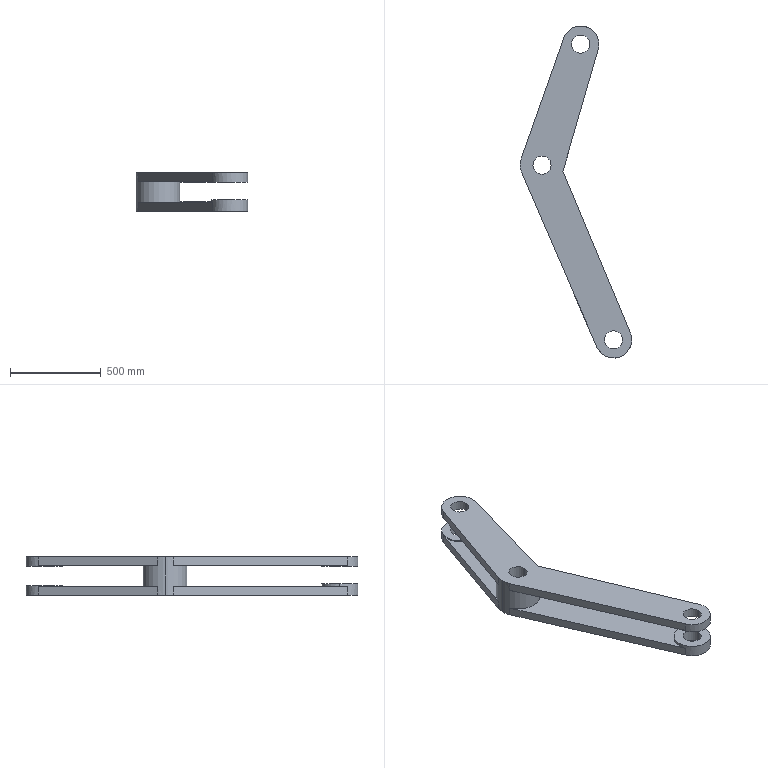Part | SolidWorks | features ICE 5, Extrusion 1 | 1 solid | 38 faces | box 614.266 x 1830 x 210 mm | volume 39335089 mm3 | cylinder 20 | plane 18 | commonest cylinder face diameters 100 x10 200 x8 240 x2
STEP:
#1=CARTESIAN_POINT('',(13655.596,320.325,-165.));
#2=VERTEX_POINT('',#1);
#3=CARTESIAN_POINT('',(13755.596,320.325,-165.));
#4=VERTEX_POINT('',#3);
#5=CARTESIAN_POINT('',(13705.596,320.325,-165.));
#6=DIRECTION('',(0.,0.,1.));
#7=DIRECTION('',(1.,0.,0.));
#8=AXIS2_PLACEMENT_3D('',#5,#6,#7);
#9=CIRCLE('',#8,50.);
#10=EDGE_CURVE('',#2,#4,#9,.T.);
#11=ORIENTED_EDGE('',*,*,#10,.F.);
#12=CARTESIAN_POINT('',(13655.596,320.325,-102.));
#13=VERTEX_POINT('',#12);
#14=CARTESIAN_POINT('',(13655.596,320.325,-165.));
#15=DIRECTION('',(0.,0.,1.));
#16=VECTOR('',#15,1000.);
#17=LINE('',#14,#16);
#18=EDGE_CURVE('',#2,#13,#17,.T.);
#19=ORIENTED_EDGE('',*,*,#18,.T.);
#20=CARTESIAN_POINT('',(13755.596,320.325,-102.));
#21=VERTEX_POINT('',#20);
#22=CARTESIAN_POINT('',(13705.596,320.325,-102.));
#23=DIRECTION('',(0.,0.,1.));
#24=DIRECTION('',(1.,0.,0.));
#25=AXIS2_PLACEMENT_3D('',#22,#23,#24);
#26=CIRCLE('',#25,50.);
#27=EDGE_CURVE('',#13,#21,#26,.T.);
#28=ORIENTED_EDGE('',*,*,#27,.T.);
#29=CARTESIAN_POINT('',(13755.596,320.325,-165.));
#30=DIRECTION('',(0.,0.,1.));
#31=VECTOR('',#30,1000.);
#32=LINE('',#29,#31);
#33=EDGE_CURVE('',#4,#21,#32,.T.);
#34=ORIENTED_EDGE('',*,*,#33,.F.);
#35=EDGE_LOOP('',(#11,#19,#28,#34));
#36=FACE_OUTER_BOUND('',#35,.T.);
#37=CARTESIAN_POINT('',(13705.596,320.325,-165.));
#38=DIRECTION('',(0.,0.,1.));
#39=DIRECTION('',(1.,0.,0.));
#40=AXIS2_PLACEMENT_3D('',#37,#38,#39);
#41=CYLINDRICAL_SURFACE('',#40,50.);
#42=ADVANCED_FACE('',(#36),#41,.F.);
#43=CARTESIAN_POINT('',(13474.67,1950.472,-165.));
#44=VERTEX_POINT('',#43);
#45=CARTESIAN_POINT('',(13574.67,1950.472,-165.));
#46=VERTEX_POINT('',#45);
#47=CARTESIAN_POINT('',(13524.67,1950.472,-165.));
#48=DIRECTION('',(0.,0.,1.));
#49=DIRECTION('',(1.,0.,0.));
#50=AXIS2_PLACEMENT_3D('',#47,#48,#49);
#51=CIRCLE('',#50,50.);
#52=EDGE_CURVE('',#44,#46,#51,.T.);
#53=ORIENTED_EDGE('',*,*,#52,.F.);
#54=CARTESIAN_POINT('',(13474.67,1950.472,-115.));
#55=VERTEX_POINT('',#54);
#56=CARTESIAN_POINT('',(13474.67,1950.472,-165.));
#57=DIRECTION('',(0.,0.,1.));
#58=VECTOR('',#57,1000.);
#59=LINE('',#56,#58);
#60=EDGE_CURVE('',#44,#55,#59,.T.);
#61=ORIENTED_EDGE('',*,*,#60,.T.);
#62=CARTESIAN_POINT('',(13574.67,1950.472,-115.));
#63=VERTEX_POINT('',#62);
#64=CARTESIAN_POINT('',(13524.67,1950.472,-115.));
#65=DIRECTION('',(0.,0.,1.));
#66=DIRECTION('',(1.,0.,0.));
#67=AXIS2_PLACEMENT_3D('',#64,#65,#66);
#68=CIRCLE('',#67,50.);
#69=EDGE_CURVE('',#55,#63,#68,.T.);
#70=ORIENTED_EDGE('',*,*,#69,.T.);
#71=CARTESIAN_POINT('',(13574.67,1950.472,-165.));
#72=DIRECTION('',(0.,0.,1.));
#73=VECTOR('',#72,1000.);
#74=LINE('',#71,#73);
#75=EDGE_CURVE('',#46,#63,#74,.T.);
#76=ORIENTED_EDGE('',*,*,#75,.F.);
#77=EDGE_LOOP('',(#53,#61,#70,#76));
#78=FACE_OUTER_BOUND('',#77,.T.);
#79=CARTESIAN_POINT('',(13524.67,1950.472,-165.));
#80=DIRECTION('',(0.,0.,1.));
#81=DIRECTION('',(1.,0.,0.));
#82=AXIS2_PLACEMENT_3D('',#79,#80,#81);
#83=CYLINDRICAL_SURFACE('',#82,50.);
#84=ADVANCED_FACE('',(#78),#83,.F.);
#85=CARTESIAN_POINT('',(13797.913,358.764,-120.));
#86=VERTEX_POINT('',#85);
#87=CARTESIAN_POINT('',(13605.596,320.325,-120.));
#88=VERTEX_POINT('',#87);
#89=CARTESIAN_POINT('',(13705.596,320.325,-120.));
#90=DIRECTION('',(0.,0.,1.));
#91=DIRECTION('',(1.,0.,0.));
#92=AXIS2_PLACEMENT_3D('',#89,#90,#91);
#93=CIRCLE('',#92,100.);
#94=EDGE_CURVE('',#86,#88,#93,.T.);
#95=ORIENTED_EDGE('',*,*,#94,.T.);
#96=CARTESIAN_POINT('',(13605.596,320.325,-102.));
#97=VERTEX_POINT('',#96);
#98=CARTESIAN_POINT('',(13605.596,320.325,-165.));
#99=DIRECTION('',(0.,0.,1.));
#100=VECTOR('',#99,1000.);
#101=LINE('',#98,#100);
#102=EDGE_CURVE('',#88,#97,#101,.T.);
#103=ORIENTED_EDGE('',*,*,#102,.T.);
#104=CARTESIAN_POINT('',(13805.596,320.325,-102.));
#105=VERTEX_POINT('',#104);
#106=CARTESIAN_POINT('',(13705.596,320.325,-102.));
#107=DIRECTION('',(0.,0.,1.));
#108=DIRECTION('',(1.,0.,0.));
#109=AXIS2_PLACEMENT_3D('',#106,#107,#108);
#110=CIRCLE('',#109,100.);
#111=EDGE_CURVE('',#105,#97,#110,.T.);
#112=ORIENTED_EDGE('',*,*,#111,.F.);
#113=CARTESIAN_POINT('',(13805.596,320.325,-165.));
#114=VERTEX_POINT('',#113);
#115=CARTESIAN_POINT('',(13805.596,320.325,-165.));
#116=DIRECTION('',(0.,0.,1.));
#117=VECTOR('',#116,1000.);
#118=LINE('',#115,#117);
#119=EDGE_CURVE('',#114,#105,#118,.T.);
#120=ORIENTED_EDGE('',*,*,#119,.F.);
#121=CARTESIAN_POINT('',(13797.913,358.764,-165.));
#122=VERTEX_POINT('',#121);
#123=CARTESIAN_POINT('',(13705.596,320.325,-165.));
#124=DIRECTION('',(0.,0.,1.));
#125=DIRECTION('',(1.,0.,0.));
#126=AXIS2_PLACEMENT_3D('',#123,#124,#125);
#127=CIRCLE('',#126,100.);
#128=EDGE_CURVE('',#114,#122,#127,.T.);
#129=ORIENTED_EDGE('',*,*,#128,.T.);
#130=CARTESIAN_POINT('',(13797.913,358.764,-165.));
#131=DIRECTION('',(0.,0.,1.));
#132=VECTOR('',#131,1000.);
#133=LINE('',#130,#132);
#134=EDGE_CURVE('',#122,#86,#133,.T.);
#135=ORIENTED_EDGE('',*,*,#134,.T.);
#136=EDGE_LOOP('',(#95,#103,#112,#120,#129,#135));
#137=FACE_OUTER_BOUND('',#136,.T.);
#138=CARTESIAN_POINT('',(13705.596,320.325,-165.));
#139=DIRECTION('',(0.,0.,1.));
#140=DIRECTION('',(1.,0.,0.));
#141=AXIS2_PLACEMENT_3D('',#138,#139,#140);
#142=CYLINDRICAL_SURFACE('',#141,100.);
#143=ADVANCED_FACE('',(#137),#142,.T.);
#144=CARTESIAN_POINT('',(13430.338,1983.658,-120.));
#145=VERTEX_POINT('',#144);
#146=CARTESIAN_POINT('',(13424.67,1950.472,-120.));
#147=VERTEX_POINT('',#146);
#148=CARTESIAN_POINT('',(13524.67,1950.472,-120.));
#149=DIRECTION('',(0.,0.,1.));
#150=DIRECTION('',(1.,0.,0.));
#151=AXIS2_PLACEMENT_3D('',#148,#149,#150);
#152=CIRCLE('',#151,100.);
#153=EDGE_CURVE('',#145,#147,#152,.T.);
#154=ORIENTED_EDGE('',*,*,#153,.T.);
#155=CARTESIAN_POINT('',(13424.67,1950.472,-115.));
#156=VERTEX_POINT('',#155);
#157=CARTESIAN_POINT('',(13424.67,1950.472,-165.));
#158=DIRECTION('',(0.,0.,1.));
#159=VECTOR('',#158,1000.);
#160=LINE('',#157,#159);
#161=EDGE_CURVE('',#147,#156,#160,.T.);
#162=ORIENTED_EDGE('',*,*,#161,.T.);
#163=CARTESIAN_POINT('',(13624.67,1950.472,-115.));
#164=VERTEX_POINT('',#163);
#165=CARTESIAN_POINT('',(13524.67,1950.472,-115.));
#166=DIRECTION('',(0.,0.,1.));
#167=DIRECTION('',(1.,0.,0.));
#168=AXIS2_PLACEMENT_3D('',#165,#166,#167);
#169=CIRCLE('',#168,100.);
#170=EDGE_CURVE('',#164,#156,#169,.T.);
#171=ORIENTED_EDGE('',*,*,#170,.F.);
#172=CARTESIAN_POINT('',(13624.67,1950.472,-165.));
#173=VERTEX_POINT('',#172);
#174=CARTESIAN_POINT('',(13624.67,1950.472,-165.));
#175=DIRECTION('',(0.,0.,1.));
#176=VECTOR('',#175,1000.);
#177=LINE('',#174,#176);
#178=EDGE_CURVE('',#173,#164,#177,.T.);
#179=ORIENTED_EDGE('',*,*,#178,.F.);
#180=CARTESIAN_POINT('',(13430.338,1983.658,-165.));
#181=VERTEX_POINT('',#180);
#182=CARTESIAN_POINT('',(13524.67,1950.472,-165.));
#183=DIRECTION('',(0.,0.,1.));
#184=DIRECTION('',(1.,0.,0.));
#185=AXIS2_PLACEMENT_3D('',#182,#183,#184);
#186=CIRCLE('',#185,100.);
#187=EDGE_CURVE('',#173,#181,#186,.T.);
#188=ORIENTED_EDGE('',*,*,#187,.T.);
#189=CARTESIAN_POINT('',(13430.338,1983.658,-165.));
#190=DIRECTION('',(0.,0.,1.));
#191=VECTOR('',#190,1000.);
#192=LINE('',#189,#191);
#193=EDGE_CURVE('',#181,#145,#192,.T.);
#194=ORIENTED_EDGE('',*,*,#193,.T.);
#195=EDGE_LOOP('',(#154,#162,#171,#179,#188,#194));
#196=FACE_OUTER_BOUND('',#195,.T.);
#197=CARTESIAN_POINT('',(13524.67,1950.472,-165.));
#198=DIRECTION('',(0.,0.,1.));
#199=DIRECTION('',(1.,0.,0.));
#200=AXIS2_PLACEMENT_3D('',#197,#198,#199);
#201=CYLINDRICAL_SURFACE('',#200,100.);
#202=ADVANCED_FACE('',(#196),#201,.T.);
#203=CARTESIAN_POINT('',(13655.596,320.325,45.));
#204=VERTEX_POINT('',#203);
#205=CARTESIAN_POINT('',(13755.596,320.325,45.));
#206=VERTEX_POINT('',#205);
#207=CARTESIAN_POINT('',(13705.596,320.325,45.));
#208=DIRECTION('',(0.,0.,1.));
#209=DIRECTION('',(1.,0.,0.));
#210=AXIS2_PLACEMENT_3D('',#207,#208,#209);
#211=CIRCLE('',#210,50.);
#212=EDGE_CURVE('',#204,#206,#211,.T.);
#213=ORIENTED_EDGE('',*,*,#212,.T.);
#214=CARTESIAN_POINT('',(13755.596,320.325,-5.));
#215=VERTEX_POINT('',#214);
#216=CARTESIAN_POINT('',(13755.596,320.325,45.));
#217=DIRECTION('',(0.,0.,-1.));
#218=VECTOR('',#217,1000.);
#219=LINE('',#216,#218);
#220=EDGE_CURVE('',#206,#215,#219,.T.);
#221=ORIENTED_EDGE('',*,*,#220,.T.);
#222=CARTESIAN_POINT('',(13655.596,320.325,-5.));
#223=VERTEX_POINT('',#222);
#224=CARTESIAN_POINT('',(13705.596,320.325,-5.));
#225=DIRECTION('',(0.,0.,1.));
#226=DIRECTION('',(1.,0.,0.));
#227=AXIS2_PLACEMENT_3D('',#224,#225,#226);
#228=CIRCLE('',#227,50.);
#229=EDGE_CURVE('',#223,#215,#228,.T.);
#230=ORIENTED_EDGE('',*,*,#229,.F.);
#231=CARTESIAN_POINT('',(13655.596,320.325,45.));
#232=DIRECTION('',(0.,0.,-1.));
#233=VECTOR('',#232,1000.);
#234=LINE('',#231,#233);
#235=EDGE_CURVE('',#204,#223,#234,.T.);
#236=ORIENTED_EDGE('',*,*,#235,.F.);
#237=EDGE_LOOP('',(#213,#221,#230,#236));
#238=FACE_OUTER_BOUND('',#237,.T.);
#239=CARTESIAN_POINT('',(13705.596,320.325,45.));
#240=DIRECTION('',(0.,0.,-1.));
#241=DIRECTION('',(-1.,0.,0.));
#242=AXIS2_PLACEMENT_3D('',#239,#240,#241);
#243=CYLINDRICAL_SURFACE('',#242,50.);
#244=ADVANCED_FACE('',(#238),#243,.F.);
#245=CARTESIAN_POINT('',(13624.67,1950.472,45.));
#246=VERTEX_POINT('',#245);
#247=CARTESIAN_POINT('',(13430.338,1983.658,45.));
#248=VERTEX_POINT('',#247);
#249=CARTESIAN_POINT('',(13524.67,1950.472,45.));
#250=DIRECTION('',(0.,0.,1.));
#251=DIRECTION('',(1.,0.,0.));
#252=AXIS2_PLACEMENT_3D('',#249,#250,#251);
#253=CIRCLE('',#252,100.);
#254=EDGE_CURVE('',#246,#248,#253,.T.);
#255=ORIENTED_EDGE('',*,*,#254,.F.);
#256=CARTESIAN_POINT('',(13624.67,1950.472,-5.));
#257=VERTEX_POINT('',#256);
#258=CARTESIAN_POINT('',(13624.67,1950.472,45.));
#259=DIRECTION('',(0.,0.,-1.));
#260=VECTOR('',#259,1000.);
#261=LINE('',#258,#260);
#262=EDGE_CURVE('',#246,#257,#261,.T.);
#263=ORIENTED_EDGE('',*,*,#262,.T.);
#264=CARTESIAN_POINT('',(13424.67,1950.472,-5.));
#265=VERTEX_POINT('',#264);
#266=CARTESIAN_POINT('',(13524.67,1950.472,-5.));
#267=DIRECTION('',(0.,0.,1.));
#268=DIRECTION('',(1.,0.,0.));
#269=AXIS2_PLACEMENT_3D('',#266,#267,#268);
#270=CIRCLE('',#269,100.);
#271=EDGE_CURVE('',#257,#265,#270,.T.);
#272=ORIENTED_EDGE('',*,*,#271,.T.);
#273=CARTESIAN_POINT('',(13424.67,1950.472,0.));
#274=VERTEX_POINT('',#273);
#275=CARTESIAN_POINT('',(13424.67,1950.472,45.));
#276=DIRECTION('',(0.,0.,-1.));
#277=VECTOR('',#276,1000.);
#278=LINE('',#275,#277);
#279=EDGE_CURVE('',#274,#265,#278,.T.);
#280=ORIENTED_EDGE('',*,*,#279,.F.);
#281=CARTESIAN_POINT('',(13430.338,1983.658,0.));
#282=VERTEX_POINT('',#281);
#283=CARTESIAN_POINT('',(13524.67,1950.472,0.));
#284=DIRECTION('',(0.,0.,1.));
#285=DIRECTION('',(1.,0.,0.));
#286=AXIS2_PLACEMENT_3D('',#283,#284,#285);
#287=CIRCLE('',#286,100.);
#288=EDGE_CURVE('',#282,#274,#287,.T.);
#289=ORIENTED_EDGE('',*,*,#288,.F.);
#290=CARTESIAN_POINT('',(13430.338,1983.658,45.));
#291=DIRECTION('',(0.,0.,-1.));
#292=VECTOR('',#291,1000.);
#293=LINE('',#290,#292);
#294=EDGE_CURVE('',#248,#282,#293,.T.);
#295=ORIENTED_EDGE('',*,*,#294,.F.);
#296=EDGE_LOOP('',(#255,#263,#272,#280,#289,#295));
#297=FACE_OUTER_BOUND('',#296,.T.);
#298=CARTESIAN_POINT('',(13524.67,1950.472,45.));
#299=DIRECTION('',(0.,0.,-1.));
#300=DIRECTION('',(-1.,0.,0.));
#301=AXIS2_PLACEMENT_3D('',#298,#299,#300);
#302=CYLINDRICAL_SURFACE('',#301,100.);
#303=ADVANCED_FACE('',(#297),#302,.T.);
#304=CARTESIAN_POINT('',(13474.67,1950.472,45.));
#305=VERTEX_POINT('',#304);
#306=CARTESIAN_POINT('',(13574.67,1950.472,45.));
#307=VERTEX_POINT('',#306);
#308=CARTESIAN_POINT('',(13524.67,1950.472,45.));
#309=DIRECTION('',(0.,0.,1.));
#310=DIRECTION('',(1.,0.,0.));
#311=AXIS2_PLACEMENT_3D('',#308,#309,#310);
#312=CIRCLE('',#311,50.);
#313=EDGE_CURVE('',#305,#307,#312,.T.);
#314=ORIENTED_EDGE('',*,*,#313,.T.);
#315=CARTESIAN_POINT('',(13574.67,1950.472,-5.));
#316=VERTEX_POINT('',#315);
#317=CARTESIAN_POINT('',(13574.67,1950.472,45.));
#318=DIRECTION('',(0.,0.,-1.));
#319=VECTOR('',#318,1000.);
#320=LINE('',#317,#319);
#321=EDGE_CURVE('',#307,#316,#320,.T.);
#322=ORIENTED_EDGE('',*,*,#321,.T.);
#323=CARTESIAN_POINT('',(13474.67,1950.472,-5.));
#324=VERTEX_POINT('',#323);
#325=CARTESIAN_POINT('',(13524.67,1950.472,-5.));
#326=DIRECTION('',(0.,0.,1.));
#327=DIRECTION('',(1.,0.,0.));
#328=AXIS2_PLACEMENT_3D('',#325,#326,#327);
#329=CIRCLE('',#328,50.);
#330=EDGE_CURVE('',#324,#316,#329,.T.);
#331=ORIENTED_EDGE('',*,*,#330,.F.);
#332=CARTESIAN_POINT('',(13474.67,1950.472,45.));
#333=DIRECTION('',(0.,0.,-1.));
#334=VECTOR('',#333,1000.);
#335=LINE('',#332,#334);
#336=EDGE_CURVE('',#305,#324,#335,.T.);
#337=ORIENTED_EDGE('',*,*,#336,.F.);
#338=EDGE_LOOP('',(#314,#322,#331,#337));
#339=FACE_OUTER_BOUND('',#338,.T.);
#340=CARTESIAN_POINT('',(13524.67,1950.472,45.));
#341=DIRECTION('',(0.,0.,-1.));
#342=DIRECTION('',(-1.,0.,0.));
#343=AXIS2_PLACEMENT_3D('',#340,#341,#342);
#344=CYLINDRICAL_SURFACE('',#343,50.);
#345=ADVANCED_FACE('',(#339),#344,.F.);
#346=CARTESIAN_POINT('',(13261.33,1283.774,45.));
#347=VERTEX_POINT('',#346);
#348=CARTESIAN_POINT('',(13361.33,1283.774,45.));
#349=VERTEX_POINT('',#348);
#350=CARTESIAN_POINT('',(13311.33,1283.774,45.));
#351=DIRECTION('',(0.,0.,1.));
#352=DIRECTION('',(1.,0.,0.));
#353=AXIS2_PLACEMENT_3D('',#350,#351,#352);
#354=CIRCLE('',#353,50.);
#355=EDGE_CURVE('',#347,#349,#354,.T.);
#356=ORIENTED_EDGE('',*,*,#355,.T.);
#357=CARTESIAN_POINT('',(13361.33,1283.774,-165.));
#358=VERTEX_POINT('',#357);
#359=CARTESIAN_POINT('',(13361.33,1283.774,45.));
#360=DIRECTION('',(0.,0.,-1.));
#361=VECTOR('',#360,1000.);
#362=LINE('',#359,#361);
#363=EDGE_CURVE('',#349,#358,#362,.T.);
#364=ORIENTED_EDGE('',*,*,#363,.T.);
#365=CARTESIAN_POINT('',(13261.33,1283.774,-165.));
#366=VERTEX_POINT('',#365);
#367=CARTESIAN_POINT('',(13311.33,1283.774,-165.));
#368=DIRECTION('',(0.,0.,1.));
#369=DIRECTION('',(1.,0.,0.));
#370=AXIS2_PLACEMENT_3D('',#367,#368,#369);
#371=CIRCLE('',#370,50.);
#372=EDGE_CURVE('',#366,#358,#371,.T.);
#373=ORIENTED_EDGE('',*,*,#372,.F.);
#374=CARTESIAN_POINT('',(13261.33,1283.774,45.));
#375=DIRECTION('',(0.,0.,-1.));
#376=VECTOR('',#375,1000.);
#377=LINE('',#374,#376);
#378=EDGE_CURVE('',#347,#366,#377,.T.);
#379=ORIENTED_EDGE('',*,*,#378,.F.);
#380=EDGE_LOOP('',(#356,#364,#373,#379));
#381=FACE_OUTER_BOUND('',#380,.T.);
#382=CARTESIAN_POINT('',(13311.33,1283.774,45.));
#383=DIRECTION('',(0.,0.,-1.));
#384=DIRECTION('',(-1.,0.,0.));
#385=AXIS2_PLACEMENT_3D('',#382,#383,#384);
#386=CYLINDRICAL_SURFACE('',#385,50.);
#387=ADVANCED_FACE('',(#381),#386,.F.);
#388=CARTESIAN_POINT('',(13805.596,320.325,45.));
#389=VERTEX_POINT('',#388);
#390=CARTESIAN_POINT('',(13797.913,358.764,45.));
#391=VERTEX_POINT('',#390);
#392=CARTESIAN_POINT('',(13705.596,320.325,45.));
#393=DIRECTION('',(0.,0.,1.));
#394=DIRECTION('',(1.,0.,0.));
#395=AXIS2_PLACEMENT_3D('',#392,#393,#394);
#396=CIRCLE('',#395,100.);
#397=EDGE_CURVE('',#389,#391,#396,.T.);
#398=ORIENTED_EDGE('',*,*,#397,.F.);
#399=CARTESIAN_POINT('',(13805.596,320.325,-5.));
#400=VERTEX_POINT('',#399);
#401=CARTESIAN_POINT('',(13805.596,320.325,45.));
#402=DIRECTION('',(0.,0.,-1.));
#403=VECTOR('',#402,1000.);
#404=LINE('',#401,#403);
#405=EDGE_CURVE('',#389,#400,#404,.T.);
#406=ORIENTED_EDGE('',*,*,#405,.T.);
#407=CARTESIAN_POINT('',(13605.596,320.325,-5.));
#408=VERTEX_POINT('',#407);
#409=CARTESIAN_POINT('',(13705.596,320.325,-5.));
#410=DIRECTION('',(0.,0.,1.));
#411=DIRECTION('',(1.,0.,0.));
#412=AXIS2_PLACEMENT_3D('',#409,#410,#411);
#413=CIRCLE('',#412,100.);
#414=EDGE_CURVE('',#400,#408,#413,.T.);
#415=ORIENTED_EDGE('',*,*,#414,.T.);
#416=CARTESIAN_POINT('',(13605.596,320.325,0.));
#417=VERTEX_POINT('',#416);
#418=CARTESIAN_POINT('',(13605.596,320.325,45.));
#419=DIRECTION('',(0.,0.,-1.));
#420=VECTOR('',#419,1000.);
#421=LINE('',#418,#420);
#422=EDGE_CURVE('',#417,#408,#421,.T.);
#423=ORIENTED_EDGE('',*,*,#422,.F.);
#424=CARTESIAN_POINT('',(13797.913,358.764,0.));
#425=VERTEX_POINT('',#424);
#426=CARTESIAN_POINT('',(13705.596,320.325,0.));
#427=DIRECTION('',(0.,0.,1.));
#428=DIRECTION('',(1.,0.,0.));
#429=AXIS2_PLACEMENT_3D('',#426,#427,#428);
#430=CIRCLE('',#429,100.);
#431=EDGE_CURVE('',#425,#417,#430,.T.);
#432=ORIENTED_EDGE('',*,*,#431,.F.);
#433=CARTESIAN_POINT('',(13797.913,358.764,45.));
#434=DIRECTION('',(0.,0.,-1.));
#435=VECTOR('',#434,1000.);
#436=LINE('',#433,#435);
#437=EDGE_CURVE('',#391,#425,#436,.T.);
#438=ORIENTED_EDGE('',*,*,#437,.F.);
#439=EDGE_LOOP('',(#398,#406,#415,#423,#432,#438));
#440=FACE_OUTER_BOUND('',#439,.T.);
#441=CARTESIAN_POINT('',(13705.596,320.325,45.));
#442=DIRECTION('',(0.,0.,-1.));
#443=DIRECTION('',(-1.,0.,0.));
#444=AXIS2_PLACEMENT_3D('',#441,#442,#443);
#445=CYLINDRICAL_SURFACE('',#444,100.);
#446=ADVANCED_FACE('',(#440),#445,.T.);
#447=CARTESIAN_POINT('',(13431.33,1283.774,0.));
#448=VERTEX_POINT('',#447);
#449=CARTESIAN_POINT('',(13198.13,1323.598,0.));
#450=VERTEX_POINT('',#449);
#451=CARTESIAN_POINT('',(13311.33,1283.774,0.));
#452=DIRECTION('',(0.,0.,1.));
#453=DIRECTION('',(1.,0.,0.));
#454=AXIS2_PLACEMENT_3D('',#451,#452,#453);
#455=CIRCLE('',#454,120.);
#456=EDGE_CURVE('',#448,#450,#455,.T.);
#457=ORIENTED_EDGE('',*,*,#456,.F.);
#458=CARTESIAN_POINT('',(13431.33,1283.774,-120.));
#459=VERTEX_POINT('',#458);
#460=CARTESIAN_POINT('',(13431.33,1283.774,45.));
#461=DIRECTION('',(0.,0.,-1.));
#462=VECTOR('',#461,1000.);
#463=LINE('',#460,#462);
#464=EDGE_CURVE('',#448,#459,#463,.T.);
#465=ORIENTED_EDGE('',*,*,#464,.T.);
#466=CARTESIAN_POINT('',(13198.13,1323.598,-120.));
#467=VERTEX_POINT('',#466);
#468=CARTESIAN_POINT('',(13311.33,1283.774,-120.));
#469=DIRECTION('',(0.,0.,1.));
#470=DIRECTION('',(1.,0.,0.));
#471=AXIS2_PLACEMENT_3D('',#468,#469,#470);
#472=CIRCLE('',#471,120.);
#473=EDGE_CURVE('',#459,#467,#472,.T.);
#474=ORIENTED_EDGE('',*,*,#473,.T.);
#475=CARTESIAN_POINT('',(13198.13,1323.598,-165.));
#476=VERTEX_POINT('',#475);
#477=CARTESIAN_POINT('',(13198.13,1323.598,-165.));
#478=DIRECTION('',(0.,0.,1.));
#479=VECTOR('',#478,1000.);
#480=LINE('',#477,#479);
#481=EDGE_CURVE('',#476,#467,#480,.T.);
#482=ORIENTED_EDGE('',*,*,#481,.F.);
#483=CARTESIAN_POINT('',(13191.33,1283.774,-165.));
#484=VERTEX_POINT('',#483);
#485=CARTESIAN_POINT('',(13311.33,1283.774,-165.));
#486=DIRECTION('',(0.,0.,1.));
#487=DIRECTION('',(1.,0.,0.));
#488=AXIS2_PLACEMENT_3D('',#485,#486,#487);
#489=CIRCLE('',#488,120.);
#490=EDGE_CURVE('',#476,#484,#489,.T.);
#491=ORIENTED_EDGE('',*,*,#490,.T.);
#492=CARTESIAN_POINT('',(13191.33,1283.774,45.));
#493=VERTEX_POINT('',#492);
#494=CARTESIAN_POINT('',(13191.33,1283.774,45.));
#495=DIRECTION('',(0.,0.,-1.));
#496=VECTOR('',#495,1000.);
#497=LINE('',#494,#496);
#498=EDGE_CURVE('',#493,#484,#497,.T.);
#499=ORIENTED_EDGE('',*,*,#498,.F.);
#500=CARTESIAN_POINT('',(13198.13,1323.598,45.));
#501=VERTEX_POINT('',#500);
#502=CARTESIAN_POINT('',(13311.33,1283.774,45.));
#503=DIRECTION('',(0.,0.,1.));
#504=DIRECTION('',(1.,0.,0.));
#505=AXIS2_PLACEMENT_3D('',#502,#503,#504);
#506=CIRCLE('',#505,120.);
#507=EDGE_CURVE('',#501,#493,#506,.T.);
#508=ORIENTED_EDGE('',*,*,#507,.F.);
#509=CARTESIAN_POINT('',(13198.13,1323.598,45.));
#510=DIRECTION('',(0.,0.,-1.));
#511=VECTOR('',#510,1000.);
#512=LINE('',#509,#511);
#513=EDGE_CURVE('',#501,#450,#512,.T.);
#514=ORIENTED_EDGE('',*,*,#513,.T.);
#515=EDGE_LOOP('',(#457,#465,#474,#482,#491,#499,#508,#514));
#516=FACE_OUTER_BOUND('',#515,.T.);
#517=CARTESIAN_POINT('',(13311.33,1283.774,45.));
#518=DIRECTION('',(0.,0.,-1.));
#519=DIRECTION('',(-1.,0.,0.));
#520=AXIS2_PLACEMENT_3D('',#517,#518,#519);
#521=CYLINDRICAL_SURFACE('',#520,120.);
#522=ADVANCED_FACE('',(#516),#521,.T.);
#523=CARTESIAN_POINT('',(13613.79,280.68,-120.));
#524=VERTEX_POINT('',#523);
#525=CARTESIAN_POINT('',(13201.163,1236.2,-120.));
#526=VERTEX_POINT('',#525);
#527=CARTESIAN_POINT('',(11576.243,4999.026,-120.));
#528=DIRECTION('',(-0.3964,0.9181,0.));
#529=VECTOR('',#528,1000.);
#530=LINE('',#527,#529);
#531=EDGE_CURVE('',#524,#526,#530,.T.);
#532=ORIENTED_EDGE('',*,*,#531,.F.);
#533=CARTESIAN_POINT('',(13705.596,320.325,-120.));
#534=DIRECTION('',(0.,0.,1.));
#535=DIRECTION('',(1.,0.,0.));
#536=AXIS2_PLACEMENT_3D('',#533,#534,#535);
#537=CIRCLE('',#536,100.);
#538=EDGE_CURVE('',#88,#524,#537,.T.);
#539=ORIENTED_EDGE('',*,*,#538,.F.);
#540=ORIENTED_EDGE('',*,*,#94,.F.);
#541=CARTESIAN_POINT('',(13426.619,1250.482,-120.));
#542=VERTEX_POINT('',#541);
#543=CARTESIAN_POINT('',(11886.503,4949.304,-120.));
#544=DIRECTION('',(0.3844,-0.9232,0.));
#545=VECTOR('',#544,1000.);
#546=LINE('',#543,#545);
#547=EDGE_CURVE('',#542,#86,#546,.T.);
#548=ORIENTED_EDGE('',*,*,#547,.F.);
#549=CARTESIAN_POINT('',(13311.33,1283.774,-120.));
#550=DIRECTION('',(0.,0.,1.));
#551=DIRECTION('',(1.,0.,0.));
#552=AXIS2_PLACEMENT_3D('',#549,#550,#551);
#553=CIRCLE('',#552,120.);
#554=EDGE_CURVE('',#526,#542,#553,.T.);
#555=ORIENTED_EDGE('',*,*,#554,.F.);
#556=EDGE_LOOP('',(#532,#539,#540,#548,#555));
#557=FACE_OUTER_BOUND('',#556,.T.);
#558=CARTESIAN_POINT('',(0.,0.,-120.));
#559=DIRECTION('',(0.,0.,1.));
#560=DIRECTION('',(1.,0.,0.));
#561=AXIS2_PLACEMENT_3D('',#558,#559,#560);
#562=PLANE('',#561);
#563=ADVANCED_FACE('',(#557),#562,.T.);
#564=CARTESIAN_POINT('',(13620.745,1922.728,-120.));
#565=VERTEX_POINT('',#564);
#566=CARTESIAN_POINT('',(12059.853,-3482.547,-120.));
#567=DIRECTION('',(-0.2774,-0.9607,0.));
#568=VECTOR('',#567,1000.);
#569=LINE('',#566,#568);
#570=EDGE_CURVE('',#565,#542,#569,.T.);
#571=ORIENTED_EDGE('',*,*,#570,.F.);
#572=CARTESIAN_POINT('',(13524.67,1950.472,-120.));
#573=DIRECTION('',(0.,0.,1.));
#574=DIRECTION('',(1.,0.,0.));
#575=AXIS2_PLACEMENT_3D('',#572,#573,#574);
#576=CIRCLE('',#575,100.);
#577=EDGE_CURVE('',#147,#565,#576,.T.);
#578=ORIENTED_EDGE('',*,*,#577,.F.);
#579=ORIENTED_EDGE('',*,*,#153,.F.);
#580=CARTESIAN_POINT('',(11330.248,-3985.948,-120.));
#581=DIRECTION('',(-0.3319,-0.9433,0.));
#582=VECTOR('',#581,1000.);
#583=LINE('',#580,#582);
#584=EDGE_CURVE('',#145,#467,#583,.T.);
#585=ORIENTED_EDGE('',*,*,#584,.T.);
#586=ORIENTED_EDGE('',*,*,#473,.F.);
#587=CARTESIAN_POINT('',(13311.33,1283.774,-120.));
#588=DIRECTION('',(0.,0.,1.));
#589=DIRECTION('',(1.,0.,0.));
#590=AXIS2_PLACEMENT_3D('',#587,#588,#589);
#591=CIRCLE('',#590,120.);
#592=EDGE_CURVE('',#542,#459,#591,.T.);
#593=ORIENTED_EDGE('',*,*,#592,.F.);
#594=EDGE_LOOP('',(#571,#578,#579,#585,#586,#593));
#595=FACE_OUTER_BOUND('',#594,.T.);
#596=CARTESIAN_POINT('',(0.,0.,-120.));
#597=DIRECTION('',(0.,0.,1.));
#598=DIRECTION('',(1.,0.,0.));
#599=AXIS2_PLACEMENT_3D('',#596,#597,#598);
#600=PLANE('',#599);
#601=ADVANCED_FACE('',(#595),#600,.T.);
#602=CARTESIAN_POINT('',(13426.619,1250.482,0.));
#603=VERTEX_POINT('',#602);
#604=CARTESIAN_POINT('',(11886.503,4949.304,0.));
#605=DIRECTION('',(0.3844,-0.9232,0.));
#606=VECTOR('',#605,1000.);
#607=LINE('',#604,#606);
#608=EDGE_CURVE('',#603,#425,#607,.T.);
#609=ORIENTED_EDGE('',*,*,#608,.T.);
#610=ORIENTED_EDGE('',*,*,#431,.T.);
#611=CARTESIAN_POINT('',(13613.79,280.68,0.));
#612=VERTEX_POINT('',#611);
#613=CARTESIAN_POINT('',(13705.596,320.325,0.));
#614=DIRECTION('',(0.,0.,1.));
#615=DIRECTION('',(1.,0.,0.));
#616=AXIS2_PLACEMENT_3D('',#613,#614,#615);
#617=CIRCLE('',#616,100.);
#618=EDGE_CURVE('',#417,#612,#617,.T.);
#619=ORIENTED_EDGE('',*,*,#618,.T.);
#620=CARTESIAN_POINT('',(13201.163,1236.2,0.));
#621=VERTEX_POINT('',#620);
#622=CARTESIAN_POINT('',(11576.243,4999.026,0.));
#623=DIRECTION('',(-0.3964,0.9181,0.));
#624=VECTOR('',#623,1000.);
#625=LINE('',#622,#624);
#626=EDGE_CURVE('',#612,#621,#625,.T.);
#627=ORIENTED_EDGE('',*,*,#626,.T.);
#628=CARTESIAN_POINT('',(13311.33,1283.774,0.));
#629=DIRECTION('',(0.,0.,1.));
#630=DIRECTION('',(1.,0.,0.));
#631=AXIS2_PLACEMENT_3D('',#628,#629,#630);
#632=CIRCLE('',#631,120.);
#633=EDGE_CURVE('',#621,#603,#632,.T.);
#634=ORIENTED_EDGE('',*,*,#633,.T.);
#635=EDGE_LOOP('',(#609,#610,#619,#627,#634));
#636=FACE_OUTER_BOUND('',#635,.T.);
#637=CARTESIAN_POINT('',(0.,0.,0.));
#638=DIRECTION('',(0.,0.,1.));
#639=DIRECTION('',(1.,0.,0.));
#640=AXIS2_PLACEMENT_3D('',#637,#638,#639);
#641=PLANE('',#640);
#642=ADVANCED_FACE('',(#636),#641,.F.);
#643=CARTESIAN_POINT('',(11330.248,-3985.948,0.));
#644=DIRECTION('',(-0.3319,-0.9433,0.));
#645=VECTOR('',#644,1000.);
#646=LINE('',#643,#645);
#647=EDGE_CURVE('',#282,#450,#646,.T.);
#648=ORIENTED_EDGE('',*,*,#647,.T.);
#649=ORIENTED_EDGE('',*,*,#513,.F.);
#650=CARTESIAN_POINT('',(11330.248,-3985.948,45.));
#651=DIRECTION('',(-0.3319,-0.9433,0.));
#652=VECTOR('',#651,1000.);
#653=LINE('',#650,#652);
#654=EDGE_CURVE('',#248,#501,#653,.T.);
#655=ORIENTED_EDGE('',*,*,#654,.F.);
#656=ORIENTED_EDGE('',*,*,#294,.T.);
#657=EDGE_LOOP('',(#648,#649,#655,#656));
#658=FACE_OUTER_BOUND('',#657,.T.);
#659=CARTESIAN_POINT('',(11330.248,-3985.948,45.));
#660=DIRECTION('',(0.9433,-0.3319,0.));
#661=DIRECTION('',(0.3319,0.9433,0.));
#662=AXIS2_PLACEMENT_3D('',#659,#660,#661);
#663=PLANE('',#662);
#664=ADVANCED_FACE('',(#658),#663,.F.);
#665=ORIENTED_EDGE('',*,*,#464,.F.);
#666=CARTESIAN_POINT('',(13311.33,1283.774,0.));
#667=DIRECTION('',(0.,0.,1.));
#668=DIRECTION('',(1.,0.,0.));
#669=AXIS2_PLACEMENT_3D('',#666,#667,#668);
#670=CIRCLE('',#669,120.);
#671=EDGE_CURVE('',#603,#448,#670,.T.);
#672=ORIENTED_EDGE('',*,*,#671,.F.);
#673=ORIENTED_EDGE('',*,*,#633,.F.);
#674=CARTESIAN_POINT('',(13201.163,1236.2,45.));
#675=VERTEX_POINT('',#674);
#676=CARTESIAN_POINT('',(13201.163,1236.2,45.));
#677=DIRECTION('',(0.,0.,-1.));
#678=VECTOR('',#677,1000.);
#679=LINE('',#676,#678);
#680=EDGE_CURVE('',#675,#621,#679,.T.);
#681=ORIENTED_EDGE('',*,*,#680,.F.);
#682=CARTESIAN_POINT('',(13311.33,1283.774,45.));
#683=DIRECTION('',(0.,0.,1.));
#684=DIRECTION('',(1.,0.,0.));
#685=AXIS2_PLACEMENT_3D('',#682,#683,#684);
#686=CIRCLE('',#685,120.);
#687=EDGE_CURVE('',#493,#675,#686,.T.);
#688=ORIENTED_EDGE('',*,*,#687,.F.);
#689=ORIENTED_EDGE('',*,*,#498,.T.);
#690=CARTESIAN_POINT('',(13201.163,1236.2,-165.));
#691=VERTEX_POINT('',#690);
#692=CARTESIAN_POINT('',(13311.33,1283.774,-165.));
#693=DIRECTION('',(0.,0.,1.));
#694=DIRECTION('',(1.,0.,0.));
#695=AXIS2_PLACEMENT_3D('',#692,#693,#694);
#696=CIRCLE('',#695,120.);
#697=EDGE_CURVE('',#484,#691,#696,.T.);
#698=ORIENTED_EDGE('',*,*,#697,.T.);
#699=CARTESIAN_POINT('',(13201.163,1236.2,-165.));
#700=DIRECTION('',(0.,0.,1.));
#701=VECTOR('',#700,1000.);
#702=LINE('',#699,#701);
#703=EDGE_CURVE('',#691,#526,#702,.T.);
#704=ORIENTED_EDGE('',*,*,#703,.T.);
#705=ORIENTED_EDGE('',*,*,#554,.T.);
#706=ORIENTED_EDGE('',*,*,#592,.T.);
#707=EDGE_LOOP('',(#665,#672,#673,#681,#688,#689,#698,#704,#705,#706));
#708=FACE_OUTER_BOUND('',#707,.T.);
#709=CARTESIAN_POINT('',(13311.33,1283.774,45.));
#710=DIRECTION('',(0.,0.,-1.));
#711=DIRECTION('',(-1.,0.,0.));
#712=AXIS2_PLACEMENT_3D('',#709,#710,#711);
#713=CYLINDRICAL_SURFACE('',#712,120.);
#714=ADVANCED_FACE('',(#708),#713,.T.);
#715=ORIENTED_EDGE('',*,*,#626,.F.);
#716=CARTESIAN_POINT('',(13613.79,280.68,45.));
#717=VERTEX_POINT('',#716);
#718=CARTESIAN_POINT('',(13613.79,280.68,45.));
#719=DIRECTION('',(0.,0.,-1.));
#720=VECTOR('',#719,1000.);
#721=LINE('',#718,#720);
#722=EDGE_CURVE('',#717,#612,#721,.T.);
#723=ORIENTED_EDGE('',*,*,#722,.F.);
#724=CARTESIAN_POINT('',(11576.243,4999.026,45.));
#725=DIRECTION('',(-0.3964,0.9181,0.));
#726=VECTOR('',#725,1000.);
#727=LINE('',#724,#726);
#728=EDGE_CURVE('',#717,#675,#727,.T.);
#729=ORIENTED_EDGE('',*,*,#728,.T.);
#730=ORIENTED_EDGE('',*,*,#680,.T.);
#731=EDGE_LOOP('',(#715,#723,#729,#730));
#732=FACE_OUTER_BOUND('',#731,.T.);
#733=CARTESIAN_POINT('',(11576.243,4999.026,45.));
#734=DIRECTION('',(-0.9181,-0.3964,0.));
#735=DIRECTION('',(0.3964,-0.9181,0.));
#736=AXIS2_PLACEMENT_3D('',#733,#734,#735);
#737=PLANE('',#736);
#738=ADVANCED_FACE('',(#732),#737,.T.);
#739=ORIENTED_EDGE('',*,*,#405,.F.);
#740=CARTESIAN_POINT('',(13705.596,320.325,45.));
#741=DIRECTION('',(0.,0.,1.));
#742=DIRECTION('',(1.,0.,0.));
#743=AXIS2_PLACEMENT_3D('',#740,#741,#742);
#744=CIRCLE('',#743,100.);
#745=EDGE_CURVE('',#717,#389,#744,.T.);
#746=ORIENTED_EDGE('',*,*,#745,.F.);
#747=ORIENTED_EDGE('',*,*,#722,.T.);
#748=ORIENTED_EDGE('',*,*,#618,.F.);
#749=ORIENTED_EDGE('',*,*,#422,.T.);
#750=CARTESIAN_POINT('',(13705.596,320.325,-5.));
#751=DIRECTION('',(0.,0.,1.));
#752=DIRECTION('',(1.,0.,0.));
#753=AXIS2_PLACEMENT_3D('',#750,#751,#752);
#754=CIRCLE('',#753,100.);
#755=EDGE_CURVE('',#408,#400,#754,.T.);
#756=ORIENTED_EDGE('',*,*,#755,.T.);
#757=EDGE_LOOP('',(#739,#746,#747,#748,#749,#756));
#758=FACE_OUTER_BOUND('',#757,.T.);
#759=CARTESIAN_POINT('',(13705.596,320.325,45.));
#760=DIRECTION('',(0.,0.,-1.));
#761=DIRECTION('',(-1.,0.,0.));
#762=AXIS2_PLACEMENT_3D('',#759,#760,#761);
#763=CYLINDRICAL_SURFACE('',#762,100.);
#764=ADVANCED_FACE('',(#758),#763,.T.);
#765=ORIENTED_EDGE('',*,*,#608,.F.);
#766=CARTESIAN_POINT('',(13426.619,1250.482,45.));
#767=VERTEX_POINT('',#766);
#768=CARTESIAN_POINT('',(13426.619,1250.482,45.));
#769=DIRECTION('',(0.,0.,-1.));
#770=VECTOR('',#769,1000.);
#771=LINE('',#768,#770);
#772=EDGE_CURVE('',#767,#603,#771,.T.);
#773=ORIENTED_EDGE('',*,*,#772,.F.);
#774=CARTESIAN_POINT('',(11886.503,4949.304,45.));
#775=DIRECTION('',(0.3844,-0.9232,0.));
#776=VECTOR('',#775,1000.);
#777=LINE('',#774,#776);
#778=EDGE_CURVE('',#767,#391,#777,.T.);
#779=ORIENTED_EDGE('',*,*,#778,.T.);
#780=ORIENTED_EDGE('',*,*,#437,.T.);
#781=EDGE_LOOP('',(#765,#773,#779,#780));
#782=FACE_OUTER_BOUND('',#781,.T.);
#783=CARTESIAN_POINT('',(11886.503,4949.304,45.));
#784=DIRECTION('',(0.9232,0.3844,0.));
#785=DIRECTION('',(-0.3844,0.9232,0.));
#786=AXIS2_PLACEMENT_3D('',#783,#784,#785);
#787=PLANE('',#786);
#788=ADVANCED_FACE('',(#782),#787,.T.);
#789=CARTESIAN_POINT('',(13620.745,1922.728,0.));
#790=VERTEX_POINT('',#789);
#791=CARTESIAN_POINT('',(12059.853,-3482.547,0.));
#792=DIRECTION('',(-0.2774,-0.9607,0.));
#793=VECTOR('',#792,1000.);
#794=LINE('',#791,#793);
#795=EDGE_CURVE('',#790,#603,#794,.T.);
#796=ORIENTED_EDGE('',*,*,#795,.F.);
#797=CARTESIAN_POINT('',(13620.745,1922.728,45.));
#798=VERTEX_POINT('',#797);
#799=CARTESIAN_POINT('',(13620.745,1922.728,45.));
#800=DIRECTION('',(0.,0.,-1.));
#801=VECTOR('',#800,1000.);
#802=LINE('',#799,#801);
#803=EDGE_CURVE('',#798,#790,#802,.T.);
#804=ORIENTED_EDGE('',*,*,#803,.F.);
#805=CARTESIAN_POINT('',(12059.853,-3482.547,45.));
#806=DIRECTION('',(-0.2774,-0.9607,0.));
#807=VECTOR('',#806,1000.);
#808=LINE('',#805,#807);
#809=EDGE_CURVE('',#798,#767,#808,.T.);
#810=ORIENTED_EDGE('',*,*,#809,.T.);
#811=ORIENTED_EDGE('',*,*,#772,.T.);
#812=EDGE_LOOP('',(#796,#804,#810,#811));
#813=FACE_OUTER_BOUND('',#812,.T.);
#814=CARTESIAN_POINT('',(12059.853,-3482.547,45.));
#815=DIRECTION('',(0.9607,-0.2774,0.));
#816=DIRECTION('',(0.2774,0.9607,0.));
#817=AXIS2_PLACEMENT_3D('',#814,#815,#816);
#818=PLANE('',#817);
#819=ADVANCED_FACE('',(#813),#818,.T.);
#820=ORIENTED_EDGE('',*,*,#363,.F.);
#821=CARTESIAN_POINT('',(13311.33,1283.774,45.));
#822=DIRECTION('',(0.,0.,1.));
#823=DIRECTION('',(1.,0.,0.));
#824=AXIS2_PLACEMENT_3D('',#821,#822,#823);
#825=CIRCLE('',#824,50.);
#826=EDGE_CURVE('',#349,#347,#825,.T.);
#827=ORIENTED_EDGE('',*,*,#826,.T.);
#828=ORIENTED_EDGE('',*,*,#378,.T.);
#829=CARTESIAN_POINT('',(13311.33,1283.774,-165.));
#830=DIRECTION('',(0.,0.,1.));
#831=DIRECTION('',(1.,0.,0.));
#832=AXIS2_PLACEMENT_3D('',#829,#830,#831);
#833=CIRCLE('',#832,50.);
#834=EDGE_CURVE('',#358,#366,#833,.T.);
#835=ORIENTED_EDGE('',*,*,#834,.F.);
#836=EDGE_LOOP('',(#820,#827,#828,#835));
#837=FACE_OUTER_BOUND('',#836,.T.);
#838=CARTESIAN_POINT('',(13311.33,1283.774,45.));
#839=DIRECTION('',(0.,0.,-1.));
#840=DIRECTION('',(-1.,0.,0.));
#841=AXIS2_PLACEMENT_3D('',#838,#839,#840);
#842=CYLINDRICAL_SURFACE('',#841,50.);
#843=ADVANCED_FACE('',(#837),#842,.F.);
#844=ORIENTED_EDGE('',*,*,#321,.F.);
#845=CARTESIAN_POINT('',(13524.67,1950.472,45.));
#846=DIRECTION('',(0.,0.,1.));
#847=DIRECTION('',(1.,0.,0.));
#848=AXIS2_PLACEMENT_3D('',#845,#846,#847);
#849=CIRCLE('',#848,50.);
#850=EDGE_CURVE('',#307,#305,#849,.T.);
#851=ORIENTED_EDGE('',*,*,#850,.T.);
#852=ORIENTED_EDGE('',*,*,#336,.T.);
#853=CARTESIAN_POINT('',(13524.67,1950.472,-5.));
#854=DIRECTION('',(0.,0.,1.));
#855=DIRECTION('',(1.,0.,0.));
#856=AXIS2_PLACEMENT_3D('',#853,#854,#855);
#857=CIRCLE('',#856,50.);
#858=EDGE_CURVE('',#316,#324,#857,.T.);
#859=ORIENTED_EDGE('',*,*,#858,.F.);
#860=EDGE_LOOP('',(#844,#851,#852,#859));
#861=FACE_OUTER_BOUND('',#860,.T.);
#862=CARTESIAN_POINT('',(13524.67,1950.472,45.));
#863=DIRECTION('',(0.,0.,-1.));
#864=DIRECTION('',(-1.,0.,0.));
#865=AXIS2_PLACEMENT_3D('',#862,#863,#864);
#866=CYLINDRICAL_SURFACE('',#865,50.);
#867=ADVANCED_FACE('',(#861),#866,.F.);
#868=ORIENTED_EDGE('',*,*,#262,.F.);
#869=CARTESIAN_POINT('',(13524.67,1950.472,45.));
#870=DIRECTION('',(0.,0.,1.));
#871=DIRECTION('',(1.,0.,0.));
#872=AXIS2_PLACEMENT_3D('',#869,#870,#871);
#873=CIRCLE('',#872,100.);
#874=EDGE_CURVE('',#798,#246,#873,.T.);
#875=ORIENTED_EDGE('',*,*,#874,.F.);
#876=ORIENTED_EDGE('',*,*,#803,.T.);
#877=CARTESIAN_POINT('',(13524.67,1950.472,0.));
#878=DIRECTION('',(0.,0.,1.));
#879=DIRECTION('',(1.,0.,0.));
#880=AXIS2_PLACEMENT_3D('',#877,#878,#879);
#881=CIRCLE('',#880,100.);
#882=EDGE_CURVE('',#274,#790,#881,.T.);
#883=ORIENTED_EDGE('',*,*,#882,.F.);
#884=ORIENTED_EDGE('',*,*,#279,.T.);
#885=CARTESIAN_POINT('',(13524.67,1950.472,-5.));
#886=DIRECTION('',(0.,0.,1.));
#887=DIRECTION('',(1.,0.,0.));
#888=AXIS2_PLACEMENT_3D('',#885,#886,#887);
#889=CIRCLE('',#888,100.);
#890=EDGE_CURVE('',#265,#257,#889,.T.);
#891=ORIENTED_EDGE('',*,*,#890,.T.);
#892=EDGE_LOOP('',(#868,#875,#876,#883,#884,#891));
#893=FACE_OUTER_BOUND('',#892,.T.);
#894=CARTESIAN_POINT('',(13524.67,1950.472,45.));
#895=DIRECTION('',(0.,0.,-1.));
#896=DIRECTION('',(-1.,0.,0.));
#897=AXIS2_PLACEMENT_3D('',#894,#895,#896);
#898=CYLINDRICAL_SURFACE('',#897,100.);
#899=ADVANCED_FACE('',(#893),#898,.T.);
#900=ORIENTED_EDGE('',*,*,#220,.F.);
#901=CARTESIAN_POINT('',(13705.596,320.325,45.));
#902=DIRECTION('',(0.,0.,1.));
#903=DIRECTION('',(1.,0.,0.));
#904=AXIS2_PLACEMENT_3D('',#901,#902,#903);
#905=CIRCLE('',#904,50.);
#906=EDGE_CURVE('',#206,#204,#905,.T.);
#907=ORIENTED_EDGE('',*,*,#906,.T.);
#908=ORIENTED_EDGE('',*,*,#235,.T.);
#909=CARTESIAN_POINT('',(13705.596,320.325,-5.));
#910=DIRECTION('',(0.,0.,1.));
#911=DIRECTION('',(1.,0.,0.));
#912=AXIS2_PLACEMENT_3D('',#909,#910,#911);
#913=CIRCLE('',#912,50.);
#914=EDGE_CURVE('',#215,#223,#913,.T.);
#915=ORIENTED_EDGE('',*,*,#914,.F.);
#916=EDGE_LOOP('',(#900,#907,#908,#915));
#917=FACE_OUTER_BOUND('',#916,.T.);
#918=CARTESIAN_POINT('',(13705.596,320.325,45.));
#919=DIRECTION('',(0.,0.,-1.));
#920=DIRECTION('',(-1.,0.,0.));
#921=AXIS2_PLACEMENT_3D('',#918,#919,#920);
#922=CYLINDRICAL_SURFACE('',#921,50.);
#923=ADVANCED_FACE('',(#917),#922,.F.);
#924=ORIENTED_EDGE('',*,*,#654,.T.);
#925=ORIENTED_EDGE('',*,*,#507,.T.);
#926=ORIENTED_EDGE('',*,*,#687,.T.);
#927=ORIENTED_EDGE('',*,*,#728,.F.);
#928=ORIENTED_EDGE('',*,*,#745,.T.);
#929=ORIENTED_EDGE('',*,*,#397,.T.);
#930=ORIENTED_EDGE('',*,*,#778,.F.);
#931=ORIENTED_EDGE('',*,*,#809,.F.);
#932=ORIENTED_EDGE('',*,*,#874,.T.);
#933=ORIENTED_EDGE('',*,*,#254,.T.);
#934=EDGE_LOOP('',(#924,#925,#926,#927,#928,#929,#930,#931,#932,#933));
#935=FACE_OUTER_BOUND('',#934,.T.);
#936=ORIENTED_EDGE('',*,*,#313,.F.);
#937=ORIENTED_EDGE('',*,*,#850,.F.);
#938=EDGE_LOOP('',(#936,#937));
#939=FACE_BOUND('',#938,.T.);
#940=ORIENTED_EDGE('',*,*,#355,.F.);
#941=ORIENTED_EDGE('',*,*,#826,.F.);
#942=EDGE_LOOP('',(#940,#941));
#943=FACE_BOUND('',#942,.T.);
#944=ORIENTED_EDGE('',*,*,#212,.F.);
#945=ORIENTED_EDGE('',*,*,#906,.F.);
#946=EDGE_LOOP('',(#944,#945));
#947=FACE_BOUND('',#946,.T.);
#948=CARTESIAN_POINT('',(0.,0.,45.));
#949=DIRECTION('',(0.,0.,1.));
#950=DIRECTION('',(1.,0.,0.));
#951=AXIS2_PLACEMENT_3D('',#948,#949,#950);
#952=PLANE('',#951);
#953=ADVANCED_FACE('',(#935,#939,#943,#947),#952,.T.);
#954=ORIENTED_EDGE('',*,*,#647,.F.);
#955=ORIENTED_EDGE('',*,*,#288,.T.);
#956=ORIENTED_EDGE('',*,*,#882,.T.);
#957=ORIENTED_EDGE('',*,*,#795,.T.);
#958=ORIENTED_EDGE('',*,*,#671,.T.);
#959=ORIENTED_EDGE('',*,*,#456,.T.);
#960=EDGE_LOOP('',(#954,#955,#956,#957,#958,#959));
#961=FACE_OUTER_BOUND('',#960,.T.);
#962=CARTESIAN_POINT('',(0.,0.,0.));
#963=DIRECTION('',(0.,0.,1.));
#964=DIRECTION('',(1.,0.,0.));
#965=AXIS2_PLACEMENT_3D('',#962,#963,#964);
#966=PLANE('',#965);
#967=ADVANCED_FACE('',(#961),#966,.F.);
#968=ORIENTED_EDGE('',*,*,#330,.T.);
#969=ORIENTED_EDGE('',*,*,#858,.T.);
#970=EDGE_LOOP('',(#968,#969));
#971=FACE_BOUND('',#970,.T.);
#972=ORIENTED_EDGE('',*,*,#890,.F.);
#973=ORIENTED_EDGE('',*,*,#271,.F.);
#974=EDGE_LOOP('',(#972,#973));
#975=FACE_OUTER_BOUND('',#974,.T.);
#976=CARTESIAN_POINT('',(0.,0.,-5.));
#977=DIRECTION('',(0.,0.,1.));
#978=DIRECTION('',(1.,0.,0.));
#979=AXIS2_PLACEMENT_3D('',#976,#977,#978);
#980=PLANE('',#979);
#981=ADVANCED_FACE('',(#971,#975),#980,.F.);
#982=ORIENTED_EDGE('',*,*,#229,.T.);
#983=ORIENTED_EDGE('',*,*,#914,.T.);
#984=EDGE_LOOP('',(#982,#983));
#985=FACE_BOUND('',#984,.T.);
#986=ORIENTED_EDGE('',*,*,#755,.F.);
#987=ORIENTED_EDGE('',*,*,#414,.F.);
#988=EDGE_LOOP('',(#986,#987));
#989=FACE_OUTER_BOUND('',#988,.T.);
#990=CARTESIAN_POINT('',(0.,0.,-5.));
#991=DIRECTION('',(0.,0.,1.));
#992=DIRECTION('',(1.,0.,0.));
#993=AXIS2_PLACEMENT_3D('',#990,#991,#992);
#994=PLANE('',#993);
#995=ADVANCED_FACE('',(#985,#989),#994,.F.);
#996=ORIENTED_EDGE('',*,*,#584,.F.);
#997=ORIENTED_EDGE('',*,*,#193,.F.);
#998=CARTESIAN_POINT('',(11330.248,-3985.948,-165.));
#999=DIRECTION('',(-0.3319,-0.9433,0.));
#1000=VECTOR('',#999,1000.);
#1001=LINE('',#998,#1000);
#1002=EDGE_CURVE('',#181,#476,#1001,.T.);
#1003=ORIENTED_EDGE('',*,*,#1002,.T.);
#1004=ORIENTED_EDGE('',*,*,#481,.T.);
#1005=EDGE_LOOP('',(#996,#997,#1003,#1004));
#1006=FACE_OUTER_BOUND('',#1005,.T.);
#1007=CARTESIAN_POINT('',(11330.248,-3985.948,-165.));
#1008=DIRECTION('',(-0.9433,0.3319,0.));
#1009=DIRECTION('',(-0.3319,-0.9433,0.));
#1010=AXIS2_PLACEMENT_3D('',#1007,#1008,#1009);
#1011=PLANE('',#1010);
#1012=ADVANCED_FACE('',(#1006),#1011,.T.);
#1013=ORIENTED_EDGE('',*,*,#161,.F.);
#1014=ORIENTED_EDGE('',*,*,#577,.T.);
#1015=CARTESIAN_POINT('',(13620.745,1922.728,-165.));
#1016=VERTEX_POINT('',#1015);
#1017=CARTESIAN_POINT('',(13620.745,1922.728,-165.));
#1018=DIRECTION('',(0.,0.,1.));
#1019=VECTOR('',#1018,1000.);
#1020=LINE('',#1017,#1019);
#1021=EDGE_CURVE('',#1016,#565,#1020,.T.);
#1022=ORIENTED_EDGE('',*,*,#1021,.F.);
#1023=CARTESIAN_POINT('',(13524.67,1950.472,-165.));
#1024=DIRECTION('',(0.,0.,1.));
#1025=DIRECTION('',(1.,0.,0.));
#1026=AXIS2_PLACEMENT_3D('',#1023,#1024,#1025);
#1027=CIRCLE('',#1026,100.);
#1028=EDGE_CURVE('',#1016,#173,#1027,.T.);
#1029=ORIENTED_EDGE('',*,*,#1028,.T.);
#1030=ORIENTED_EDGE('',*,*,#178,.T.);
#1031=CARTESIAN_POINT('',(13524.67,1950.472,-115.));
#1032=DIRECTION('',(0.,0.,1.));
#1033=DIRECTION('',(1.,0.,0.));
#1034=AXIS2_PLACEMENT_3D('',#1031,#1032,#1033);
#1035=CIRCLE('',#1034,100.);
#1036=EDGE_CURVE('',#156,#164,#1035,.T.);
#1037=ORIENTED_EDGE('',*,*,#1036,.F.);
#1038=EDGE_LOOP('',(#1013,#1014,#1022,#1029,#1030,#1037));
#1039=FACE_OUTER_BOUND('',#1038,.T.);
#1040=CARTESIAN_POINT('',(13524.67,1950.472,-165.));
#1041=DIRECTION('',(0.,0.,1.));
#1042=DIRECTION('',(1.,0.,0.));
#1043=AXIS2_PLACEMENT_3D('',#1040,#1041,#1042);
#1044=CYLINDRICAL_SURFACE('',#1043,100.);
#1045=ADVANCED_FACE('',(#1039),#1044,.T.);
#1046=ORIENTED_EDGE('',*,*,#570,.T.);
#1047=CARTESIAN_POINT('',(13426.619,1250.482,-165.));
#1048=VERTEX_POINT('',#1047);
#1049=CARTESIAN_POINT('',(13426.619,1250.482,-165.));
#1050=DIRECTION('',(0.,0.,1.));
#1051=VECTOR('',#1050,1000.);
#1052=LINE('',#1049,#1051);
#1053=EDGE_CURVE('',#1048,#542,#1052,.T.);
#1054=ORIENTED_EDGE('',*,*,#1053,.F.);
#1055=CARTESIAN_POINT('',(12059.853,-3482.547,-165.));
#1056=DIRECTION('',(-0.2774,-0.9607,0.));
#1057=VECTOR('',#1056,1000.);
#1058=LINE('',#1055,#1057);
#1059=EDGE_CURVE('',#1016,#1048,#1058,.T.);
#1060=ORIENTED_EDGE('',*,*,#1059,.F.);
#1061=ORIENTED_EDGE('',*,*,#1021,.T.);
#1062=EDGE_LOOP('',(#1046,#1054,#1060,#1061));
#1063=FACE_OUTER_BOUND('',#1062,.T.);
#1064=CARTESIAN_POINT('',(12059.853,-3482.547,-165.));
#1065=DIRECTION('',(-0.9607,0.2774,0.));
#1066=DIRECTION('',(-0.2774,-0.9607,0.));
#1067=AXIS2_PLACEMENT_3D('',#1064,#1065,#1066);
#1068=PLANE('',#1067);
#1069=ADVANCED_FACE('',(#1063),#1068,.F.);
#1070=ORIENTED_EDGE('',*,*,#547,.T.);
#1071=ORIENTED_EDGE('',*,*,#134,.F.);
#1072=CARTESIAN_POINT('',(11886.503,4949.304,-165.));
#1073=DIRECTION('',(0.3844,-0.9232,0.));
#1074=VECTOR('',#1073,1000.);
#1075=LINE('',#1072,#1074);
#1076=EDGE_CURVE('',#1048,#122,#1075,.T.);
#1077=ORIENTED_EDGE('',*,*,#1076,.F.);
#1078=ORIENTED_EDGE('',*,*,#1053,.T.);
#1079=EDGE_LOOP('',(#1070,#1071,#1077,#1078));
#1080=FACE_OUTER_BOUND('',#1079,.T.);
#1081=CARTESIAN_POINT('',(11886.503,4949.304,-165.));
#1082=DIRECTION('',(-0.9232,-0.3844,0.));
#1083=DIRECTION('',(0.3844,-0.9232,0.));
#1084=AXIS2_PLACEMENT_3D('',#1081,#1082,#1083);
#1085=PLANE('',#1084);
#1086=ADVANCED_FACE('',(#1080),#1085,.F.);
#1087=ORIENTED_EDGE('',*,*,#102,.F.);
#1088=ORIENTED_EDGE('',*,*,#538,.T.);
#1089=CARTESIAN_POINT('',(13613.79,280.68,-165.));
#1090=VERTEX_POINT('',#1089);
#1091=CARTESIAN_POINT('',(13613.79,280.68,-165.));
#1092=DIRECTION('',(0.,0.,1.));
#1093=VECTOR('',#1092,1000.);
#1094=LINE('',#1091,#1093);
#1095=EDGE_CURVE('',#1090,#524,#1094,.T.);
#1096=ORIENTED_EDGE('',*,*,#1095,.F.);
#1097=CARTESIAN_POINT('',(13705.596,320.325,-165.));
#1098=DIRECTION('',(0.,0.,1.));
#1099=DIRECTION('',(1.,0.,0.));
#1100=AXIS2_PLACEMENT_3D('',#1097,#1098,#1099);
#1101=CIRCLE('',#1100,100.);
#1102=EDGE_CURVE('',#1090,#114,#1101,.T.);
#1103=ORIENTED_EDGE('',*,*,#1102,.T.);
#1104=ORIENTED_EDGE('',*,*,#119,.T.);
#1105=CARTESIAN_POINT('',(13705.596,320.325,-102.));
#1106=DIRECTION('',(0.,0.,1.));
#1107=DIRECTION('',(1.,0.,0.));
#1108=AXIS2_PLACEMENT_3D('',#1105,#1106,#1107);
#1109=CIRCLE('',#1108,100.);
#1110=EDGE_CURVE('',#97,#105,#1109,.T.);
#1111=ORIENTED_EDGE('',*,*,#1110,.F.);
#1112=EDGE_LOOP('',(#1087,#1088,#1096,#1103,#1104,#1111));
#1113=FACE_OUTER_BOUND('',#1112,.T.);
#1114=CARTESIAN_POINT('',(13705.596,320.325,-165.));
#1115=DIRECTION('',(0.,0.,1.));
#1116=DIRECTION('',(1.,0.,0.));
#1117=AXIS2_PLACEMENT_3D('',#1114,#1115,#1116);
#1118=CYLINDRICAL_SURFACE('',#1117,100.);
#1119=ADVANCED_FACE('',(#1113),#1118,.T.);
#1120=ORIENTED_EDGE('',*,*,#531,.T.);
#1121=ORIENTED_EDGE('',*,*,#703,.F.);
#1122=CARTESIAN_POINT('',(11576.243,4999.026,-165.));
#1123=DIRECTION('',(-0.3964,0.9181,0.));
#1124=VECTOR('',#1123,1000.);
#1125=LINE('',#1122,#1124);
#1126=EDGE_CURVE('',#1090,#691,#1125,.T.);
#1127=ORIENTED_EDGE('',*,*,#1126,.F.);
#1128=ORIENTED_EDGE('',*,*,#1095,.T.);
#1129=EDGE_LOOP('',(#1120,#1121,#1127,#1128));
#1130=FACE_OUTER_BOUND('',#1129,.T.);
#1131=CARTESIAN_POINT('',(11576.243,4999.026,-165.));
#1132=DIRECTION('',(0.9181,0.3964,0.));
#1133=DIRECTION('',(-0.3964,0.9181,0.));
#1134=AXIS2_PLACEMENT_3D('',#1131,#1132,#1133);
#1135=PLANE('',#1134);
#1136=ADVANCED_FACE('',(#1130),#1135,.F.);
#1137=ORIENTED_EDGE('',*,*,#60,.F.);
#1138=CARTESIAN_POINT('',(13524.67,1950.472,-165.));
#1139=DIRECTION('',(0.,0.,1.));
#1140=DIRECTION('',(1.,0.,0.));
#1141=AXIS2_PLACEMENT_3D('',#1138,#1139,#1140);
#1142=CIRCLE('',#1141,50.);
#1143=EDGE_CURVE('',#46,#44,#1142,.T.);
#1144=ORIENTED_EDGE('',*,*,#1143,.F.);
#1145=ORIENTED_EDGE('',*,*,#75,.T.);
#1146=CARTESIAN_POINT('',(13524.67,1950.472,-115.));
#1147=DIRECTION('',(0.,0.,1.));
#1148=DIRECTION('',(1.,0.,0.));
#1149=AXIS2_PLACEMENT_3D('',#1146,#1147,#1148);
#1150=CIRCLE('',#1149,50.);
#1151=EDGE_CURVE('',#63,#55,#1150,.T.);
#1152=ORIENTED_EDGE('',*,*,#1151,.T.);
#1153=EDGE_LOOP('',(#1137,#1144,#1145,#1152));
#1154=FACE_OUTER_BOUND('',#1153,.T.);
#1155=CARTESIAN_POINT('',(13524.67,1950.472,-165.));
#1156=DIRECTION('',(0.,0.,1.));
#1157=DIRECTION('',(1.,0.,0.));
#1158=AXIS2_PLACEMENT_3D('',#1155,#1156,#1157);
#1159=CYLINDRICAL_SURFACE('',#1158,50.);
#1160=ADVANCED_FACE('',(#1154),#1159,.F.);
#1161=ORIENTED_EDGE('',*,*,#18,.F.);
#1162=CARTESIAN_POINT('',(13705.596,320.325,-165.));
#1163=DIRECTION('',(0.,0.,1.));
#1164=DIRECTION('',(1.,0.,0.));
#1165=AXIS2_PLACEMENT_3D('',#1162,#1163,#1164);
#1166=CIRCLE('',#1165,50.);
#1167=EDGE_CURVE('',#4,#2,#1166,.T.);
#1168=ORIENTED_EDGE('',*,*,#1167,.F.);
#1169=ORIENTED_EDGE('',*,*,#33,.T.);
#1170=CARTESIAN_POINT('',(13705.596,320.325,-102.));
#1171=DIRECTION('',(0.,0.,1.));
#1172=DIRECTION('',(1.,0.,0.));
#1173=AXIS2_PLACEMENT_3D('',#1170,#1171,#1172);
#1174=CIRCLE('',#1173,50.);
#1175=EDGE_CURVE('',#21,#13,#1174,.T.);
#1176=ORIENTED_EDGE('',*,*,#1175,.T.);
#1177=EDGE_LOOP('',(#1161,#1168,#1169,#1176));
#1178=FACE_OUTER_BOUND('',#1177,.T.);
#1179=CARTESIAN_POINT('',(13705.596,320.325,-165.));
#1180=DIRECTION('',(0.,0.,1.));
#1181=DIRECTION('',(1.,0.,0.));
#1182=AXIS2_PLACEMENT_3D('',#1179,#1180,#1181);
#1183=CYLINDRICAL_SURFACE('',#1182,50.);
#1184=ADVANCED_FACE('',(#1178),#1183,.F.);
#1185=ORIENTED_EDGE('',*,*,#1002,.F.);
#1186=ORIENTED_EDGE('',*,*,#187,.F.);
#1187=ORIENTED_EDGE('',*,*,#1028,.F.);
#1188=ORIENTED_EDGE('',*,*,#1059,.T.);
#1189=ORIENTED_EDGE('',*,*,#1076,.T.);
#1190=ORIENTED_EDGE('',*,*,#128,.F.);
#1191=ORIENTED_EDGE('',*,*,#1102,.F.);
#1192=ORIENTED_EDGE('',*,*,#1126,.T.);
#1193=ORIENTED_EDGE('',*,*,#697,.F.);
#1194=ORIENTED_EDGE('',*,*,#490,.F.);
#1195=EDGE_LOOP('',(#1185,#1186,#1187,#1188,#1189,#1190,#1191,#1192,#1193,#1194));
#1196=FACE_OUTER_BOUND('',#1195,.T.);
#1197=ORIENTED_EDGE('',*,*,#1143,.T.);
#1198=ORIENTED_EDGE('',*,*,#52,.T.);
#1199=EDGE_LOOP('',(#1197,#1198));
#1200=FACE_BOUND('',#1199,.T.);
#1201=ORIENTED_EDGE('',*,*,#372,.T.);
#1202=ORIENTED_EDGE('',*,*,#834,.T.);
#1203=EDGE_LOOP('',(#1201,#1202));
#1204=FACE_BOUND('',#1203,.T.);
#1205=ORIENTED_EDGE('',*,*,#1167,.T.);
#1206=ORIENTED_EDGE('',*,*,#10,.T.);
#1207=EDGE_LOOP('',(#1205,#1206));
#1208=FACE_BOUND('',#1207,.T.);
#1209=CARTESIAN_POINT('',(0.,0.,-165.));
#1210=DIRECTION('',(0.,0.,1.));
#1211=DIRECTION('',(1.,0.,0.));
#1212=AXIS2_PLACEMENT_3D('',#1209,#1210,#1211);
#1213=PLANE('',#1212);
#1214=ADVANCED_FACE('',(#1196,#1200,#1204,#1208),#1213,.F.);
#1215=ORIENTED_EDGE('',*,*,#1151,.F.);
#1216=ORIENTED_EDGE('',*,*,#69,.F.);
#1217=EDGE_LOOP('',(#1215,#1216));
#1218=FACE_BOUND('',#1217,.T.);
#1219=ORIENTED_EDGE('',*,*,#170,.T.);
#1220=ORIENTED_EDGE('',*,*,#1036,.T.);
#1221=EDGE_LOOP('',(#1219,#1220));
#1222=FACE_OUTER_BOUND('',#1221,.T.);
#1223=CARTESIAN_POINT('',(0.,0.,-115.));
#1224=DIRECTION('',(0.,0.,1.));
#1225=DIRECTION('',(1.,0.,0.));
#1226=AXIS2_PLACEMENT_3D('',#1223,#1224,#1225);
#1227=PLANE('',#1226);
#1228=ADVANCED_FACE('',(#1218,#1222),#1227,.T.);
#1229=ORIENTED_EDGE('',*,*,#1175,.F.);
#1230=ORIENTED_EDGE('',*,*,#27,.F.);
#1231=EDGE_LOOP('',(#1229,#1230));
#1232=FACE_BOUND('',#1231,.T.);
#1233=ORIENTED_EDGE('',*,*,#111,.T.);
#1234=ORIENTED_EDGE('',*,*,#1110,.T.);
#1235=EDGE_LOOP('',(#1233,#1234));
#1236=FACE_OUTER_BOUND('',#1235,.T.);
#1237=CARTESIAN_POINT('',(0.,0.,-102.));
#1238=DIRECTION('',(0.,0.,1.));
#1239=DIRECTION('',(1.,0.,0.));
#1240=AXIS2_PLACEMENT_3D('',#1237,#1238,#1239);
#1241=PLANE('',#1240);
#1242=ADVANCED_FACE('',(#1232,#1236),#1241,.T.);
#1243=CLOSED_SHELL('',(#42,#84,#143,#202,#244,#303,#345,#387,#446,#522,#563,#601,#642,#664,#714,#738,#764,#788,#819,#843,#867,#899,#923,#953,#967,#981,#995,#1012,#1045,#1069,#1086,#1119,#1136,#1160,#1184,#1214,#1228,#1242));
#1244=MANIFOLD_SOLID_BREP('',#1243);
#1245=CARTESIAN_POINT('',(0.,0.,0.));
#1246=DIRECTION('',(0.,0.,1.));
#1247=DIRECTION('',(1.,0.,0.));
#1248=AXIS2_PLACEMENT_3D('',#1245,#1246,#1247);
#1249=(LENGTH_UNIT()NAMED_UNIT(*)SI_UNIT(.MILLI.,.METRE.));
#1250=UNCERTAINTY_MEASURE_WITH_UNIT(LENGTH_MEASURE(0.00001),#1249,'','');
#1251=(NAMED_UNIT(*)PLANE_ANGLE_UNIT()SI_UNIT($,.RADIAN.));
#1252=(NAMED_UNIT(*)SI_UNIT($,.STERADIAN.)SOLID_ANGLE_UNIT());
#1253=(GEOMETRIC_REPRESENTATION_CONTEXT(3)GLOBAL_UNCERTAINTY_ASSIGNED_CONTEXT((#1250))GLOBAL_UNIT_ASSIGNED_CONTEXT((#1249,#1251,#1252))REPRESENTATION_CONTEXT('',''));
#1254=ADVANCED_BREP_SHAPE_REPRESENTATION('',(#1244,#1248),#1253);